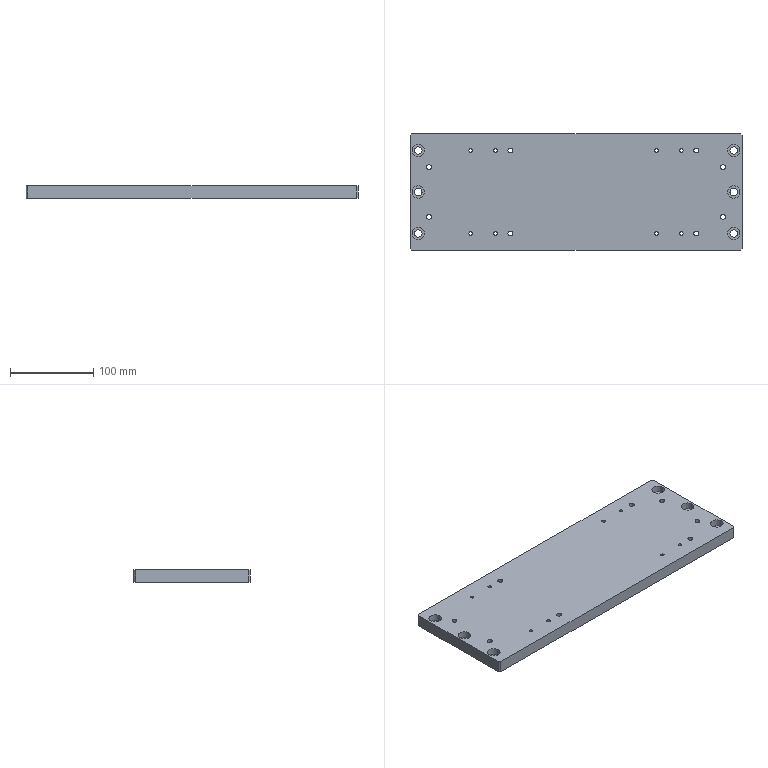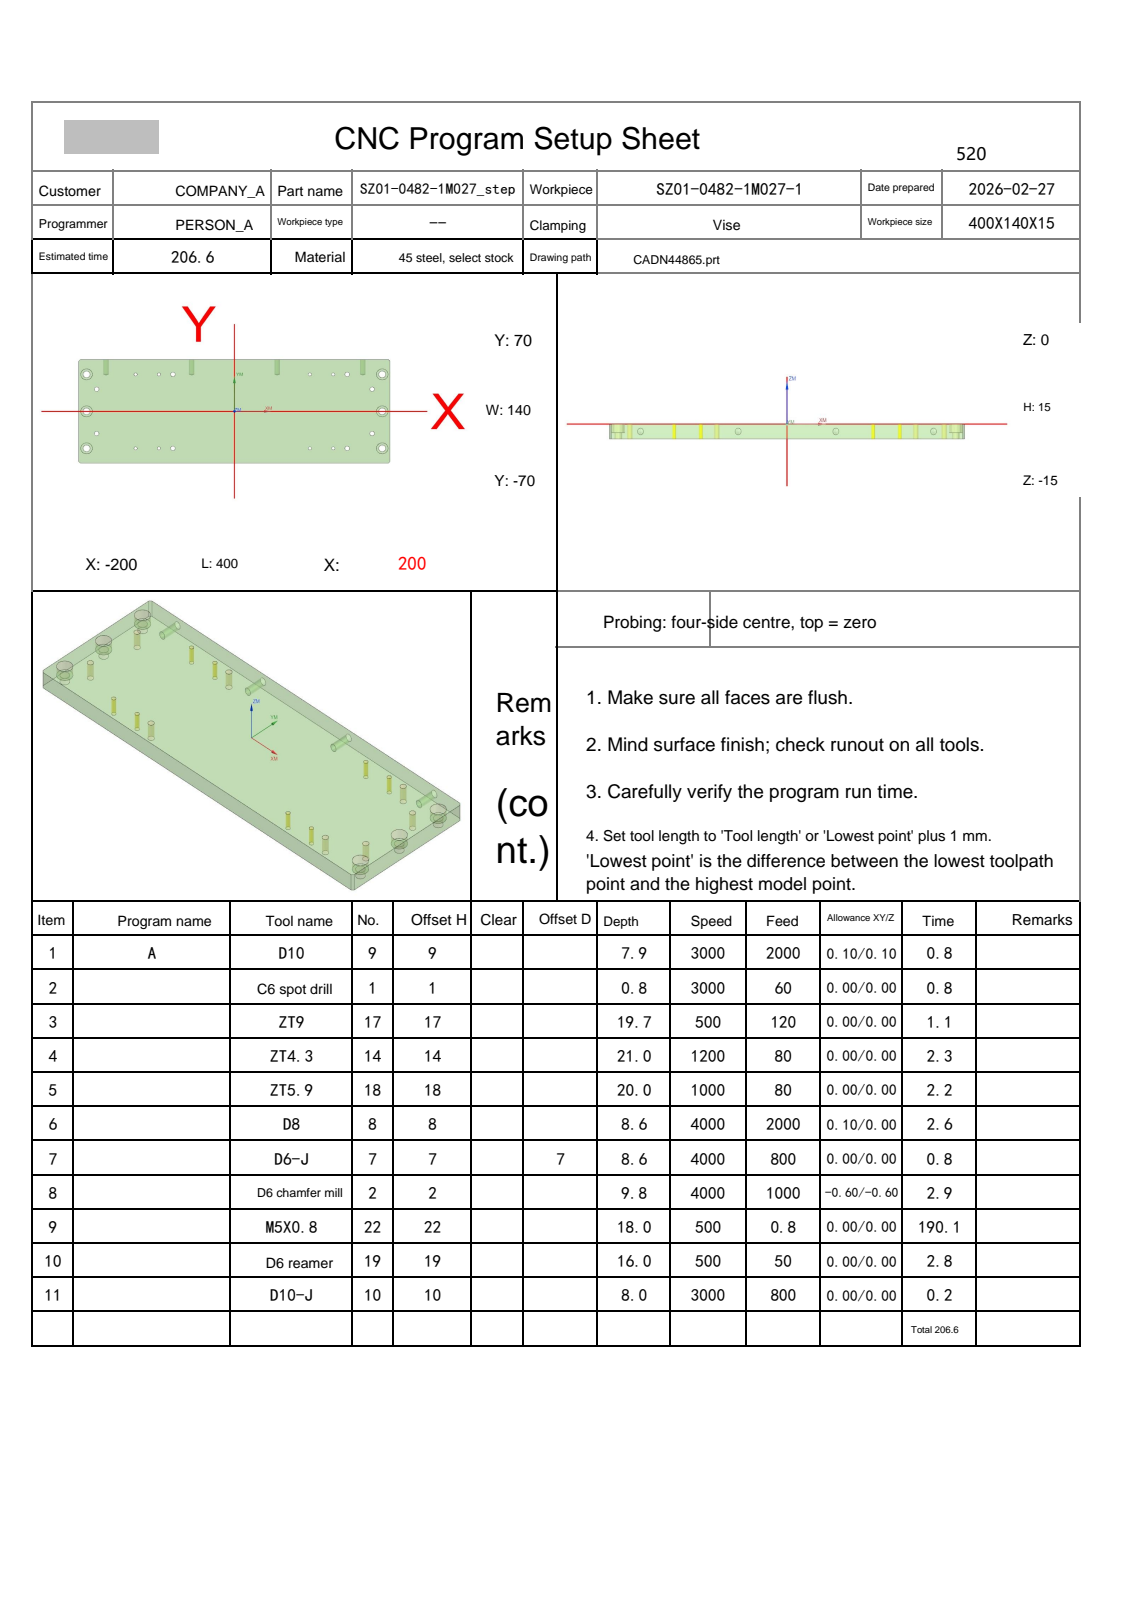NC program | NX | posted by the shop | part box 400 x 140 x 15 mm
Whole program:
%
O0001
(Machine time: 388.35 MIN)
(===Total Tool:11===)
(T9=D10     D=10.  R=0.   D-  H09 Z=-7.9  )
(T1=C6 spot drill   D=6.   R=0.   D-  H01 Z=-0.8  )
(T17=ZT9    D=9.   DR_a=118 D-  H17 Z=-19.7 )
(T14=ZT4.3  D=4.3  DR_a=118 D-  H14 Z=-21.  )
(T18=ZT5.9  D=5.9  DR_a=120 D-  H18 Z=-20.  )
(T8=D8      D=8.   R=0.   D-  H08 Z=-8.6  )
(T7=D6-J    D=6.   R=0.   D7  H07 Z=-8.6  )
(T2=D6 chamfer mill   D=6.   R=0.   D-  H02 Z=-9.8  )
(T22=M5X0.8 D=4.2  DR_a=180 D-  H22 Z=-18.  )
(T19=D6 reamer   D=6.   DR_a=180 D-  H19 Z=-16.  )
(T10=D10-J  D=10.  R=0.   D-  H10 Z=-8.   )
G80 G90 G17 G49 G40
G91 G28 Z0
M01
N1 T09 M06
(D10  D=10. R=0. H=09 ce=0.10 di=0.10)
G00 G90 G54 X195.242 Y79.97 M03 S3000
G43 H09 Z50.
M08
Z-.5
G01 X201.606 Y73.606 F2000.
X203.606 Y71.606
X209.97 Y65.242
G00 Z-1.
G01 X203.606 Y71.606
X201.606 Y73.606
X195.242 Y79.97
G00 Z-1.5
G01 X201.606 Y73.606
X203.606 Y71.606
X209.97 Y65.242
G00 Z-2.
G01 X203.606 Y71.606
X201.606 Y73.606
X195.242 Y79.97
G00 Z-2.5
G01 X201.606 Y73.606
X203.606 Y71.606
X209.97 Y65.242
G00 Z-3.
G01 X203.606 Y71.606
X201.606 Y73.606
X195.242 Y79.97
G00 Z-3.5
G01 X201.606 Y73.606
X203.606 Y71.606
X209.97 Y65.242
G00 Z-4.
G01 X203.606 Y71.606
X201.606 Y73.606
X195.242 Y79.97
G00 Z-4.5
G01 X201.606 Y73.606
X203.606 Y71.606
X209.97 Y65.242
G00 Z-5.
G01 X203.606 Y71.606
X201.606 Y73.606
X195.242 Y79.97
G00 Z-5.5
G01 X201.606 Y73.606
X203.606 Y71.606
X209.97 Y65.242
G00 Z-6.
G01 X203.606 Y71.606
X201.606 Y73.606
X195.242 Y79.97
G00 Z-6.5
G01 X201.606 Y73.606
X203.606 Y71.606
X209.97 Y65.242
G00 Z-7.
G01 X203.606 Y71.606
X201.606 Y73.606
X195.242 Y79.97
G00 Z-7.5
G01 X201.606 Y73.606
X203.606 Y71.606
X209.97 Y65.242
G00 Z-7.9
G01 X203.606 Y71.606
X201.606 Y73.606
X195.242 Y79.97
G00 Z50.
X209.97 Y-65.242
Z-.5
G01 X203.606 Y-71.606
X201.606 Y-73.606
X195.242 Y-79.97
G00 Z-1.
G01 X201.606 Y-73.606
X203.606 Y-71.606
X209.97 Y-65.242
G00 Z-1.5
G01 X203.606 Y-71.606
X201.606 Y-73.606
X195.242 Y-79.97
G00 Z-2.
G01 X201.606 Y-73.606
X203.606 Y-71.606
X209.97 Y-65.242
G00 Z-2.5
G01 X203.606 Y-71.606
X201.606 Y-73.606
X195.242 Y-79.97
G00 Z-3.
G01 X201.606 Y-73.606
X203.606 Y-71.606
X209.97 Y-65.242
G00 Z-3.5
G01 X203.606 Y-71.606
X201.606 Y-73.606
X195.242 Y-79.97
G00 Z-4.
G01 X201.606 Y-73.606
X203.606 Y-71.606
X209.97 Y-65.242
G00 Z-4.5
G01 X203.606 Y-71.606
X201.606 Y-73.606
X195.242 Y-79.97
G00 Z-5.
G01 X201.606 Y-73.606
X203.606 Y-71.606
X209.97 Y-65.242
G00 Z-5.5
G01 X203.606 Y-71.606
X201.606 Y-73.606
X195.242 Y-79.97
G00 Z-6.
G01 X201.606 Y-73.606
X203.606 Y-71.606
X209.97 Y-65.242
G00 Z-6.5
G01 X203.606 Y-71.606
X201.606 Y-73.606
X195.242 Y-79.97
G00 Z-7.
G01 X201.606 Y-73.606
X203.606 Y-71.606
X209.97 Y-65.242
G00 Z-7.5
G01 X203.606 Y-71.606
X201.606 Y-73.606
X195.242 Y-79.97
G00 Z-7.9
G01 X201.606 Y-73.606
X203.606 Y-71.606
X209.97 Y-65.242
G00 Z50.
X-195.242 Y-79.97
Z-.5
G01 X-201.606 Y-73.606
X-203.606 Y-71.606
X-209.97 Y-65.242
G00 Z-1.
G01 X-203.606 Y-71.606
X-201.606 Y-73.606
X-195.242 Y-79.97
G00 Z-1.5
G01 X-201.606 Y-73.606
X-203.606 Y-71.606
X-209.97 Y-65.242
G00 Z-2.
G01 X-203.606 Y-71.606
X-201.606 Y-73.606
X-195.242 Y-79.97
G00 Z-2.5
G01 X-201.606 Y-73.606
X-203.606 Y-71.606
X-209.97 Y-65.242
G00 Z-3.
G01 X-203.606 Y-71.606
X-201.606 Y-73.606
X-195.242 Y-79.97
G00 Z-3.5
G01 X-201.606 Y-73.606
X-203.606 Y-71.606
X-209.97 Y-65.242
G00 Z-4.
G01 X-203.606 Y-71.606
X-201.606 Y-73.606
X-195.242 Y-79.97
G00 Z-4.5
G01 X-201.606 Y-73.606
X-203.606 Y-71.606
X-209.97 Y-65.242
G00 Z-5.
G01 X-203.606 Y-71.606
X-201.606 Y-73.606
X-195.242 Y-79.97
G00 Z-5.5
G01 X-201.606 Y-73.606
X-203.606 Y-71.606
X-209.97 Y-65.242
G00 Z-6.
G01 X-203.606 Y-71.606
X-201.606 Y-73.606
X-195.242 Y-79.97
G00 Z-6.5
G01 X-201.606 Y-73.606
X-203.606 Y-71.606
X-209.97 Y-65.242
G00 Z-7.
G01 X-203.606 Y-71.606
X-201.606 Y-73.606
X-195.242 Y-79.97
G00 Z-7.5
G01 X-201.606 Y-73.606
X-203.606 Y-71.606
X-209.97 Y-65.242
G00 Z-7.9
G01 X-203.606 Y-71.606
X-201.606 Y-73.606
X-195.242 Y-79.97
G00 Z50.
X-209.97 Y65.242
Z-.5
G01 X-203.606 Y71.606
X-201.606 Y73.606
X-195.242 Y79.97
G00 Z-1.
G01 X-201.606 Y73.606
X-203.606 Y71.606
X-209.97 Y65.242
G00 Z-1.5
G01 X-203.606 Y71.606
X-201.606 Y73.606
X-195.242 Y79.97
G00 Z-2.
G01 X-201.606 Y73.606
X-203.606 Y71.606
X-209.97 Y65.242
G00 Z-2.5
G01 X-203.606 Y71.606
X-201.606 Y73.606
X-195.242 Y79.97
G00 Z-3.
G01 X-201.606 Y73.606
X-203.606 Y71.606
X-209.97 Y65.242
G00 Z-3.5
G01 X-203.606 Y71.606
X-201.606 Y73.606
X-195.242 Y79.97
G00 Z-4.
G01 X-201.606 Y73.606
X-203.606 Y71.606
X-209.97 Y65.242
G00 Z-4.5
G01 X-203.606 Y71.606
X-201.606 Y73.606
X-195.242 Y79.97
G00 Z-5.
G01 X-201.606 Y73.606
X-203.606 Y71.606
X-209.97 Y65.242
G00 Z-5.5
G01 X-203.606 Y71.606
X-201.606 Y73.606
X-195.242 Y79.97
G00 Z-6.
G01 X-201.606 Y73.606
X-203.606 Y71.606
X-209.97 Y65.242
G00 Z-6.5
G01 X-203.606 Y71.606
X-201.606 Y73.606
X-195.242 Y79.97
G00 Z-7.
G01 X-201.606 Y73.606
X-203.606 Y71.606
X-209.97 Y65.242
G00 Z-7.5
G01 X-203.606 Y71.606
X-201.606 Y73.606
X-195.242 Y79.97
G00 Z-7.9
G01 X-201.606 Y73.606
X-203.606 Y71.606
X-209.97 Y65.242
G00 Z50.
G91 G28 Z0.0
M05
M09
G91 G28 Z0.0
M01
N2 T01 M06
(C6 spot drill  D=6. R=0. H=01 ce=0.00 di=0.10)
G00 G90 G54 X97. Y50. M03 S3000
G43 H01 Z50.
M08
G98 G81 X97. Y50. Z-.8 R1. F60.
X127.
X145.
X190.
X177. Y30.
X190. Y0.0
X177. Y-30.
X190. Y-50.
X145.
X127.
X97.
X-79.
X-97.
X-127.
X-190.
X-177. Y-30.
X-190. Y0.0
X-177. Y30.
X-190. Y50.
X-127.
X-97.
X-79.
G80
G00 Z50.
G91 G28 Z0.0
M05
M09
G91 G28 Z0.0
M01
N3 T17 M06
(ZT9 D=9. DR_a=118 H=17)
G00 G90 G54 X-190. Y-50. M03 S500
G43 H17 Z50.
M08
G98 G83 X-190. Y-50. Z-19.704 R1. F120. Q2.
Y0.0
Y50.
X190.
Y0.0
Y-50.
G80
G00 Z50.
G91 G28 Z0.0
M05
M09
G91 G28 Z0.0
M01
N4 T14 M06
(ZT4.3 D=4.3 DR_a=118 H=14)
G00 G90 G54 X97. Y-50. M03 S1200
G43 H14 Z50.
M08
G98 G83 X97. Y-50. Z-21. R1. F80. Q1.5
X127.
Y50.
X97.
X-97.
X-127.
Y-50.
X-97.
G80
G00 Z50.
G91 G28 Z0.0
M05
M09
G91 G28 Z0.0
M01
N5 T18 M06
(ZT5.9 D=5.9 DR_a=120 H=18)
G00 G90 G54 X145. Y-50. M03 S1000
G43 H18 Z50.
M08
G98 G83 X145. Y-50. Z-20. R1. F80. Q1.
X177. Y-30.
Y30.
X145. Y50.
X-79.
Y-50.
X-177. Y-30.
Y30.
G80
G00 Z50.
G91 G28 Z0.0
M05
M09
G91 G28 Z0.0
M01
N6 T08 M06
(D8  D=8. R=0. H=08 ce=0.10 di=0.00)
G00 G90 G54 X190. Y0.0 M03 S4000
G43 H08 Z50.
M08
Z.5
G03 X191.7 Y-1.7 I1.7 J0.0 F2000.
X193.4 Y0.0 I0.0 J1.7
X193.4 Y0.0 Z.25 I-3.4 J0.0
X193.4 Y0.0 Z0.0 I-3.4 J0.0
X193.4 Y0.0 Z-.25 I-3.4 J0.0
X193.4 Y0.0 Z-.5 I-3.4 J0.0
X193.4 Y0.0 Z-.75 I-3.4 J0.0
X193.4 Y0.0 Z-1. I-3.4 J0.0
X193.4 Y0.0 Z-1.25 I-3.4 J0.0
X193.4 Y0.0 Z-1.5 I-3.4 J0.0
X193.4 Y0.0 Z-1.75 I-3.4 J0.0
X193.4 Y0.0 Z-2. I-3.4 J0.0
X193.4 Y0.0 Z-2.25 I-3.4 J0.0
X193.4 Y0.0 Z-2.5 I-3.4 J0.0
X193.4 Y0.0 Z-2.75 I-3.4 J0.0
X193.4 Y0.0 Z-3. I-3.4 J0.0
X193.4 Y0.0 Z-3.25 I-3.4 J0.0
X193.4 Y0.0 Z-3.5 I-3.4 J0.0
X193.4 Y0.0 Z-3.75 I-3.4 J0.0
X193.4 Y0.0 Z-4. I-3.4 J0.0
X193.4 Y0.0 Z-4.25 I-3.4 J0.0
X193.4 Y0.0 Z-4.5 I-3.4 J0.0
X193.4 Y0.0 Z-4.75 I-3.4 J0.0
X193.4 Y0.0 Z-5. I-3.4 J0.0
X193.4 Y0.0 Z-5.25 I-3.4 J0.0
X193.4 Y0.0 Z-5.5 I-3.4 J0.0
X193.4 Y0.0 Z-5.75 I-3.4 J0.0
X193.4 Y0.0 Z-6. I-3.4 J0.0
X193.4 Y0.0 Z-6.25 I-3.4 J0.0
X193.4 Y0.0 Z-6.5 I-3.4 J0.0
X193.4 Y0.0 Z-6.75 I-3.4 J0.0
X193.4 Y0.0 Z-7. I-3.4 J0.0
X193.4 Y0.0 Z-7.25 I-3.4 J0.0
X193.4 Y0.0 Z-7.5 I-3.4 J0.0
X193.4 Y0.0 Z-7.75 I-3.4 J0.0
X193.4 Y0.0 Z-8. I-3.4 J0.0
X193.4 Y0.0 Z-8.25 I-3.4 J0.0
X193.4 Y0.0 Z-8.5 I-3.4 J0.0
X187.249 Y1.998 Z-8.6 I-3.4 J0.0
X186.6 Y0.0 I2.751 J-1.998
X190. Y-3.4 I3.4 J0.0
X193.4 Y0.0 I0.0 J3.4
X190. Y3.4 I-3.4 J0.0
X187.249 Y1.998 I0.0 J-3.4
X186.925 Y.999 I1.375 J-.999
X188.625 Y-.701 I1.7 J0.0
X190. Y0.0 I0.0 J1.7
G00 Z50.
Y-50.
Z.5
G03 X191.7 Y-51.7 I1.7 J0.0
X193.4 Y-50. I0.0 J1.7
X193.4 Y-50. Z.25 I-3.4 J0.0
X193.4 Y-50. Z0.0 I-3.4 J0.0
X193.4 Y-50. Z-.25 I-3.4 J0.0
X193.4 Y-50. Z-.5 I-3.4 J0.0
X193.4 Y-50. Z-.75 I-3.4 J0.0
X193.4 Y-50. Z-1. I-3.4 J0.0
X193.4 Y-50. Z-1.25 I-3.4 J0.0
X193.4 Y-50. Z-1.5 I-3.4 J0.0
X193.4 Y-50. Z-1.75 I-3.4 J0.0
X193.4 Y-50. Z-2. I-3.4 J0.0
X193.4 Y-50. Z-2.25 I-3.4 J0.0
X193.4 Y-50. Z-2.5 I-3.4 J0.0
X193.4 Y-50. Z-2.75 I-3.4 J0.0
X193.4 Y-50. Z-3. I-3.4 J0.0
X193.4 Y-50. Z-3.25 I-3.4 J0.0
X193.4 Y-50. Z-3.5 I-3.4 J0.0
X193.4 Y-50. Z-3.75 I-3.4 J0.0
X193.4 Y-50. Z-4. I-3.4 J0.0
X193.4 Y-50. Z-4.25 I-3.4 J0.0
X193.4 Y-50. Z-4.5 I-3.4 J0.0
X193.4 Y-50. Z-4.75 I-3.4 J0.0
X193.4 Y-50. Z-5. I-3.4 J0.0
X193.4 Y-50. Z-5.25 I-3.4 J0.0
X193.4 Y-50. Z-5.5 I-3.4 J0.0
X193.4 Y-50. Z-5.75 I-3.4 J0.0
X193.4 Y-50. Z-6. I-3.4 J0.0
X193.4 Y-50. Z-6.25 I-3.4 J0.0
X193.4 Y-50. Z-6.5 I-3.4 J0.0
X193.4 Y-50. Z-6.75 I-3.4 J0.0
X193.4 Y-50. Z-7. I-3.4 J0.0
X193.4 Y-50. Z-7.25 I-3.4 J0.0
X193.4 Y-50. Z-7.5 I-3.4 J0.0
X193.4 Y-50. Z-7.75 I-3.4 J0.0
X193.4 Y-50. Z-8. I-3.4 J0.0
X193.4 Y-50. Z-8.25 I-3.4 J0.0
X193.4 Y-50. Z-8.5 I-3.4 J0.0
X187.249 Y-48.002 Z-8.6 I-3.4 J0.0
X186.6 Y-50. I2.751 J-1.998
X190. Y-53.4 I3.4 J0.0
X193.4 Y-50. I0.0 J3.4
X190. Y-46.6 I-3.4 J0.0
X187.249 Y-48.002 I0.0 J-3.4
X186.925 Y-49.001 I1.375 J-.999
X188.625 Y-50.701 I1.7 J0.0
X190. Y-50. I0.0 J1.7
G00 Z50.
Y50.
Z.5
G03 X191.7 Y48.3 I1.7 J0.0
X193.4 Y50. I0.0 J1.7
X193.4 Y50. Z.25 I-3.4 J0.0
X193.4 Y50. Z0.0 I-3.4 J0.0
X193.4 Y50. Z-.25 I-3.4 J0.0
X193.4 Y50. Z-.5 I-3.4 J0.0
X193.4 Y50. Z-.75 I-3.4 J0.0
X193.4 Y50. Z-1. I-3.4 J0.0
X193.4 Y50. Z-1.25 I-3.4 J0.0
X193.4 Y50. Z-1.5 I-3.4 J0.0
X193.4 Y50. Z-1.75 I-3.4 J0.0
X193.4 Y50. Z-2. I-3.4 J0.0
X193.4 Y50. Z-2.25 I-3.4 J0.0
X193.4 Y50. Z-2.5 I-3.4 J0.0
X193.4 Y50. Z-2.75 I-3.4 J0.0
X193.4 Y50. Z-3. I-3.4 J0.0
X193.4 Y50. Z-3.25 I-3.4 J0.0
X193.4 Y50. Z-3.5 I-3.4 J0.0
X193.4 Y50. Z-3.75 I-3.4 J0.0
X193.4 Y50. Z-4. I-3.4 J0.0
X193.4 Y50. Z-4.25 I-3.4 J0.0
X193.4 Y50. Z-4.5 I-3.4 J0.0
X193.4 Y50. Z-4.75 I-3.4 J0.0
X193.4 Y50. Z-5. I-3.4 J0.0
X193.4 Y50. Z-5.25 I-3.4 J0.0
X193.4 Y50. Z-5.5 I-3.4 J0.0
X193.4 Y50. Z-5.75 I-3.4 J0.0
X193.4 Y50. Z-6. I-3.4 J0.0
X193.4 Y50. Z-6.25 I-3.4 J0.0
X193.4 Y50. Z-6.5 I-3.4 J0.0
X193.4 Y50. Z-6.75 I-3.4 J0.0
X193.4 Y50. Z-7. I-3.4 J0.0
X193.4 Y50. Z-7.25 I-3.4 J0.0
X193.4 Y50. Z-7.5 I-3.4 J0.0
X193.4 Y50. Z-7.75 I-3.4 J0.0
X193.4 Y50. Z-8. I-3.4 J0.0
X193.4 Y50. Z-8.25 I-3.4 J0.0
X193.4 Y50. Z-8.5 I-3.4 J0.0
X187.249 Y51.998 Z-8.6 I-3.4 J0.0
X186.6 Y50. I2.751 J-1.998
X190. Y46.6 I3.4 J0.0
X193.4 Y50. I0.0 J3.4
X190. Y53.4 I-3.4 J0.0
X187.249 Y51.998 I0.0 J-3.4
X186.925 Y50.999 I1.375 J-.999
X188.625 Y49.299 I1.7 J0.0
X190. Y50. I0.0 J1.7
G00 Z50.
X-190.
Z.5
G03 X-188.3 Y48.3 I1.7 J0.0
X-186.6 Y50. I0.0 J1.7
X-186.6 Y50. Z.25 I-3.4 J0.0
X-186.6 Y50. Z0.0 I-3.4 J0.0
X-186.6 Y50. Z-.25 I-3.4 J0.0
X-186.6 Y50. Z-.5 I-3.4 J0.0
X-186.6 Y50. Z-.75 I-3.4 J0.0
X-186.6 Y50. Z-1. I-3.4 J0.0
X-186.6 Y50. Z-1.25 I-3.4 J0.0
X-186.6 Y50. Z-1.5 I-3.4 J0.0
X-186.6 Y50. Z-1.75 I-3.4 J0.0
X-186.6 Y50. Z-2. I-3.4 J0.0
X-186.6 Y50. Z-2.25 I-3.4 J0.0
X-186.6 Y50. Z-2.5 I-3.4 J0.0
X-186.6 Y50. Z-2.75 I-3.4 J0.0
X-186.6 Y50. Z-3. I-3.4 J0.0
X-186.6 Y50. Z-3.25 I-3.4 J0.0
X-186.6 Y50. Z-3.5 I-3.4 J0.0
X-186.6 Y50. Z-3.75 I-3.4 J0.0
X-186.6 Y50. Z-4. I-3.4 J0.0
X-186.6 Y50. Z-4.25 I-3.4 J0.0
X-186.6 Y50. Z-4.5 I-3.4 J0.0
X-186.6 Y50. Z-4.75 I-3.4 J0.0
X-186.6 Y50. Z-5. I-3.4 J0.0
X-186.6 Y50. Z-5.25 I-3.4 J0.0
X-186.6 Y50. Z-5.5 I-3.4 J0.0
X-186.6 Y50. Z-5.75 I-3.4 J0.0
X-186.6 Y50. Z-6. I-3.4 J0.0
X-186.6 Y50. Z-6.25 I-3.4 J0.0
X-186.6 Y50. Z-6.5 I-3.4 J0.0
X-186.6 Y50. Z-6.75 I-3.4 J0.0
X-186.6 Y50. Z-7. I-3.4 J0.0
X-186.6 Y50. Z-7.25 I-3.4 J0.0
X-186.6 Y50. Z-7.5 I-3.4 J0.0
X-186.6 Y50. Z-7.75 I-3.4 J0.0
X-186.6 Y50. Z-8. I-3.4 J0.0
X-186.6 Y50. Z-8.25 I-3.4 J0.0
X-186.6 Y50. Z-8.5 I-3.4 J0.0
X-192.751 Y51.998 Z-8.6 I-3.4 J0.0
X-193.4 Y50. I2.751 J-1.998
X-190. Y46.6 I3.4 J0.0
X-186.6 Y50. I0.0 J3.4
X-190. Y53.4 I-3.4 J0.0
X-192.751 Y51.998 I0.0 J-3.4
X-193.075 Y50.999 I1.375 J-.999
X-191.375 Y49.299 I1.7 J0.0
X-190. Y50. I0.0 J1.7
G00 Z50.
Y0.0
Z.5
G03 X-188.3 Y-1.7 I1.7 J0.0
X-186.6 Y0.0 I0.0 J1.7
X-186.6 Y0.0 Z.25 I-3.4 J0.0
X-186.6 Y0.0 Z0.0 I-3.4 J0.0
X-186.6 Y0.0 Z-.25 I-3.4 J0.0
X-186.6 Y0.0 Z-.5 I-3.4 J0.0
X-186.6 Y0.0 Z-.75 I-3.4 J0.0
X-186.6 Y0.0 Z-1. I-3.4 J0.0
X-186.6 Y0.0 Z-1.25 I-3.4 J0.0
X-186.6 Y0.0 Z-1.5 I-3.4 J0.0
X-186.6 Y0.0 Z-1.75 I-3.4 J0.0
X-186.6 Y0.0 Z-2. I-3.4 J0.0
X-186.6 Y0.0 Z-2.25 I-3.4 J0.0
X-186.6 Y0.0 Z-2.5 I-3.4 J0.0
X-186.6 Y0.0 Z-2.75 I-3.4 J0.0
X-186.6 Y0.0 Z-3. I-3.4 J0.0
X-186.6 Y0.0 Z-3.25 I-3.4 J0.0
X-186.6 Y0.0 Z-3.5 I-3.4 J0.0
X-186.6 Y0.0 Z-3.75 I-3.4 J0.0
X-186.6 Y0.0 Z-4. I-3.4 J0.0
X-186.6 Y0.0 Z-4.25 I-3.4 J0.0
X-186.6 Y0.0 Z-4.5 I-3.4 J0.0
X-186.6 Y0.0 Z-4.75 I-3.4 J0.0
X-186.6 Y0.0 Z-5. I-3.4 J0.0
X-186.6 Y0.0 Z-5.25 I-3.4 J0.0
X-186.6 Y0.0 Z-5.5 I-3.4 J0.0
X-186.6 Y0.0 Z-5.75 I-3.4 J0.0
X-186.6 Y0.0 Z-6. I-3.4 J0.0
X-186.6 Y0.0 Z-6.25 I-3.4 J0.0
X-186.6 Y0.0 Z-6.5 I-3.4 J0.0
X-186.6 Y0.0 Z-6.75 I-3.4 J0.0
X-186.6 Y0.0 Z-7. I-3.4 J0.0
X-186.6 Y0.0 Z-7.25 I-3.4 J0.0
X-186.6 Y0.0 Z-7.5 I-3.4 J0.0
X-186.6 Y0.0 Z-7.75 I-3.4 J0.0
X-186.6 Y0.0 Z-8. I-3.4 J0.0
X-186.6 Y0.0 Z-8.25 I-3.4 J0.0
X-186.6 Y0.0 Z-8.5 I-3.4 J0.0
X-192.751 Y1.998 Z-8.6 I-3.4 J0.0
X-193.4 Y0.0 I2.751 J-1.998
X-190. Y-3.4 I3.4 J0.0
X-186.6 Y0.0 I0.0 J3.4
X-190. Y3.4 I-3.4 J0.0
X-192.751 Y1.998 I0.0 J-3.4
X-193.075 Y.999 I1.375 J-.999
X-191.375 Y-.701 I1.7 J0.0
X-190. Y0.0 I0.0 J1.7
G00 Z50.
Y-50.
Z.5
G03 X-188.3 Y-51.7 I1.7 J0.0
X-186.6 Y-50. I0.0 J1.7
X-186.6 Y-50. Z.25 I-3.4 J0.0
X-186.6 Y-50. Z0.0 I-3.4 J0.0
X-186.6 Y-50. Z-.25 I-3.4 J0.0
X-186.6 Y-50. Z-.5 I-3.4 J0.0
X-186.6 Y-50. Z-.75 I-3.4 J0.0
X-186.6 Y-50. Z-1. I-3.4 J0.0
X-186.6 Y-50. Z-1.25 I-3.4 J0.0
X-186.6 Y-50. Z-1.5 I-3.4 J0.0
X-186.6 Y-50. Z-1.75 I-3.4 J0.0
X-186.6 Y-50. Z-2. I-3.4 J0.0
X-186.6 Y-50. Z-2.25 I-3.4 J0.0
X-186.6 Y-50. Z-2.5 I-3.4 J0.0
X-186.6 Y-50. Z-2.75 I-3.4 J0.0
X-186.6 Y-50. Z-3. I-3.4 J0.0
X-186.6 Y-50. Z-3.25 I-3.4 J0.0
X-186.6 Y-50. Z-3.5 I-3.4 J0.0
X-186.6 Y-50. Z-3.75 I-3.4 J0.0
X-186.6 Y-50. Z-4. I-3.4 J0.0
X-186.6 Y-50. Z-4.25 I-3.4 J0.0
X-186.6 Y-50. Z-4.5 I-3.4 J0.0
X-186.6 Y-50. Z-4.75 I-3.4 J0.0
X-186.6 Y-50. Z-5. I-3.4 J0.0
X-186.6 Y-50. Z-5.25 I-3.4 J0.0
X-186.6 Y-50. Z-5.5 I-3.4 J0.0
X-186.6 Y-50. Z-5.75 I-3.4 J0.0
X-186.6 Y-50. Z-6. I-3.4 J0.0
X-186.6 Y-50. Z-6.25 I-3.4 J0.0
X-186.6 Y-50. Z-6.5 I-3.4 J0.0
X-186.6 Y-50. Z-6.75 I-3.4 J0.0
X-186.6 Y-50. Z-7. I-3.4 J0.0
X-186.6 Y-50. Z-7.25 I-3.4 J0.0
X-186.6 Y-50. Z-7.5 I-3.4 J0.0
X-186.6 Y-50. Z-7.75 I-3.4 J0.0
X-186.6 Y-50. Z-8. I-3.4 J0.0
X-186.6 Y-50. Z-8.25 I-3.4 J0.0
X-186.6 Y-50. Z-8.5 I-3.4 J0.0
X-192.751 Y-48.002 Z-8.6 I-3.4 J0.0
X-193.4 Y-50. I2.751 J-1.998
X-190. Y-53.4 I3.4 J0.0
X-186.6 Y-50. I0.0 J3.4
X-190. Y-46.6 I-3.4 J0.0
X-192.751 Y-48.002 I0.0 J-3.4
X-193.075 Y-49.001 I1.375 J-.999
X-191.375 Y-50.701 I1.7 J0.0
X-190. Y-50. I0.0 J1.7
G00 Z50.
G91 G28 Z0.0
M05
M09
G91 G28 Z0.0
M01
N7 T07 M06
(D6-J  D=6. R=0. H=07 ce=0.00 di=0.00)
G00 G90 G54 X190. Y0.0 M03 S4000
G43 H07 Z50.
M08
Z.5
G41 D07
G01 X190.794 Y-1.153 F800.
G03 X192.468 Y-2.032 I1.674 J1.153
X194.5 Y0.0 I0.0 J2.032
X194.5 Y0.0 Z-4.5 I-4.5 J0.0
X191.916 Y-4.072 Z-8.6 I-4.5 J0.0
X194.5 Y0.0 I-1.916 J4.072
X190. Y4.5 I-4.5 J0.0
X185.5 Y0.0 I0.0 J-4.5
X190. Y-4.5 I4.5 J0.0
X191.916 Y-4.072 I0.0 J4.5
X193.083 Y-2.233 I-.865 J1.839
X191.381 Y-.228 I-2.032 J0.0
G01 G40 X190. Y0.0
G00 Z50.
Y-50.
Z.5
G41 D07
G01 X190.794 Y-51.153
G03 X192.468 Y-52.032 I1.674 J1.153
X194.5 Y-50. I0.0 J2.032
X194.5 Y-50. Z-4.5 I-4.5 J0.0
X191.916 Y-54.072 Z-8.6 I-4.5 J0.0
X194.5 Y-50. I-1.916 J4.072
X190. Y-45.5 I-4.5 J0.0
X185.5 Y-50. I0.0 J-4.5
X190. Y-54.5 I4.5 J0.0
X191.916 Y-54.072 I0.0 J4.5
X193.083 Y-52.233 I-.865 J1.839
X191.381 Y-50.228 I-2.032 J0.0
G01 G40 X190. Y-50.
G00 Z50.
Y50.
Z.5
G41 D07
G01 X190.794 Y48.847
G03 X192.468 Y47.968 I1.674 J1.153
X194.5 Y50. I0.0 J2.032
X194.5 Y50. Z-4.5 I-4.5 J0.0
X191.916 Y45.928 Z-8.6 I-4.5 J0.0
X194.5 Y50. I-1.916 J4.072
X190. Y54.5 I-4.5 J0.0
X185.5 Y50. I0.0 J-4.5
X190. Y45.5 I4.5 J0.0
X191.916 Y45.928 I0.0 J4.5
X193.083 Y47.767 I-.865 J1.839
X191.381 Y49.772 I-2.032 J0.0
G01 G40 X190. Y50.
G00 Z50.
X-190.
Z.5
G41 D07
G01 X-189.206 Y48.847
G03 X-187.532 Y47.968 I1.674 J1.153
X-185.5 Y50. I0.0 J2.032
X-185.5 Y50. Z-4.5 I-4.5 J0.0
X-188.084 Y45.928 Z-8.6 I-4.5 J0.0
X-185.5 Y50. I-1.916 J4.072
X-190. Y54.5 I-4.5 J0.0
X-194.5 Y50. I0.0 J-4.5
X-190. Y45.5 I4.5 J0.0
X-188.084 Y45.928 I0.0 J4.5
X-186.917 Y47.767 I-.865 J1.839
X-188.619 Y49.772 I-2.032 J0.0
G01 G40 X-190. Y50.
G00 Z50.
Y0.0
Z.5
G41 D07
G01 X-189.206 Y-1.153
G03 X-187.532 Y-2.032 I1.674 J1.153
X-185.5 Y0.0 I0.0 J2.032
X-185.5 Y0.0 Z-4.5 I-4.5 J0.0
X-188.084 Y-4.072 Z-8.6 I-4.5 J0.0
X-185.5 Y0.0 I-1.916 J4.072
X-190. Y4.5 I-4.5 J0.0
X-194.5 Y0.0 I0.0 J-4.5
X-190. Y-4.5 I4.5 J0.0
X-188.084 Y-4.072 I0.0 J4.5
X-186.917 Y-2.233 I-.865 J1.839
X-188.619 Y-.228 I-2.032 J0.0
G01 G40 X-190. Y0.0
G00 Z50.
Y-50.
Z.5
G41 D07
G01 X-189.206 Y-51.153
G03 X-187.532 Y-52.032 I1.674 J1.153
X-185.5 Y-50. I0.0 J2.032
X-185.5 Y-50. Z-4.5 I-4.5 J0.0
X-188.084 Y-54.072 Z-8.6 I-4.5 J0.0
X-185.5 Y-50. I-1.916 J4.072
X-190. Y-45.5 I-4.5 J0.0
X-194.5 Y-50. I0.0 J-4.5
X-190. Y-54.5 I4.5 J0.0
X-188.084 Y-54.072 I0.0 J4.5
X-186.917 Y-52.233 I-.865 J1.839
X-188.619 Y-50.228 I-2.032 J0.0
G01 G40 X-190. Y-50.
G00 Z50.
G91 G28 Z0.0
M05
M09
G91 G28 Z0.0
M01
N8 T02 M06
(D6 chamfer mill  D=6. R=0. H=02 ce=-0.60 di=0.00)
G00 G90 G54 X-97.093 Y-49.306 M03 S4000
G43 H02 Z50.
M08
Z-.5
G01 Z-1. F200.
X-97.2 Y-48.5
G03 X-98.7 Y-50. I0.0 J-1.5
X-97. Y-51.7 I1.7 J0.0
X-95.3 Y-50. I0.0 J1.7
X-97. Y-48.3 I-1.7 J0.0
X-98.7 Y-50. I0.0 J-1.7
X-97.2 Y-51.5 I1.5 J0.0
G01 X-97.093 Y-50.694
Z-.5
G00 Z50.
X-127.093 Y-49.306
Z-.5
G01 Z-1.
X-127.2 Y-48.5
G03 X-128.7 Y-50. I0.0 J-1.5
X-127. Y-51.7 I1.7 J0.0
X-125.3 Y-50. I0.0 J1.7
X-127. Y-48.3 I-1.7 J0.0
X-128.7 Y-50. I0.0 J-1.7
X-127.2 Y-51.5 I1.5 J0.0
G01 X-127.093 Y-50.694
Z-.5
G00 Z50.
Y50.694
Z-.5
G01 Z-1.
X-127.2 Y51.5
G03 X-128.7 Y50. I0.0 J-1.5
X-127. Y48.3 I1.7 J0.0
X-125.3 Y50. I0.0 J1.7
X-127. Y51.7 I-1.7 J0.0
X-128.7 Y50. I0.0 J-1.7
X-127.2 Y48.5 I1.5 J0.0
G01 X-127.093 Y49.306
Z-.5
G00 Z50.
X-97.093 Y50.694
Z-.5
G01 Z-1.
X-97.2 Y51.5
G03 X-98.7 Y50. I0.0 J-1.5
X-97. Y48.3 I1.7 J0.0
X-95.3 Y50. I0.0 J1.7
X-97. Y51.7 I-1.7 J0.0
X-98.7 Y50. I0.0 J-1.7
X-97.2 Y48.5 I1.5 J0.0
G01 X-97.093 Y49.306
Z-.5
G00 Z50.
X96.907 Y50.694
Z-.5
G01 Z-1.
X96.8 Y51.5
G03 X95.3 Y50. I0.0 J-1.5
X97. Y48.3 I1.7 J0.0
X98.7 Y50. I0.0 J1.7
X97. Y51.7 I-1.7 J0.0
X95.3 Y50. I0.0 J-1.7
X96.8 Y48.5 I1.5 J0.0
G01 X96.907 Y49.306
Z-.5
G00 Z50.
X126.907 Y50.694
Z-.5
G01 Z-1.
X126.8 Y51.5
G03 X125.3 Y50. I0.0 J-1.5
X127. Y48.3 I1.7 J0.0
X128.7 Y50. I0.0 J1.7
X127. Y51.7 I-1.7 J0.0
X125.3 Y50. I0.0 J-1.7
X126.8 Y48.5 I1.5 J0.0
G01 X126.907 Y49.306
Z-.5
G00 Z50.
Y-49.306
Z-.5
G01 Z-1.
X126.8 Y-48.5
G03 X125.3 Y-50. I0.0 J-1.5
X127. Y-51.7 I1.7 J0.0
X128.7 Y-50. I0.0 J1.7
X127. Y-48.3 I-1.7 J0.0
X125.3 Y-50. I0.0 J-1.7
X126.8 Y-51.5 I1.5 J0.0
G01 X126.907 Y-50.694
Z-.5
G00 Z50.
X96.907 Y-49.306
Z-.5
G01 Z-1.
X96.8 Y-48.5
G03 X95.3 Y-50. I0.0 J-1.5
X97. Y-51.7 I1.7 J0.0
X98.7 Y-50. I0.0 J1.7
X97. Y-48.3 I-1.7 J0.0
X95.3 Y-50. I0.0 J-1.7
X96.8 Y-51.5 I1.5 J0.0
G01 X96.907 Y-50.694
Z-.5
G00 Z50.
G00 G90 X-.386 Y71.227 M03 S3500
Z50.
Z.172
G01 Z-1.2 F1000.
G03 X-.1 Y71.027 I1.286 J1.532
G01 X-.054 Y70.997
X0.0 Y71.
X198.
X198.259 Y70.966
X198.5 Y70.866
X198.707 Y70.707
X200.707 Y68.707
X200.866 Y68.5
X200.966 Y68.259
X201. Y68.
Y-68.
X200.966 Y-68.259
X200.866 Y-68.5
X200.707 Y-68.707
X198.707 Y-70.707
X198.5 Y-70.866
X198.259 Y-70.966
X198. Y-71.
X-198.
X-198.259 Y-70.966
X-198.5 Y-70.866
X-198.707 Y-70.707
X-200.707 Y-68.707
X-200.866 Y-68.5
X-200.966 Y-68.259
X-201. Y-68.
Y68.
X-200.966 Y68.259
X-200.866 Y68.5
X-200.707 Y68.707
X-198.707 Y70.707
X-198.5 Y70.866
X-198.259 Y70.966
X-198. Y71.
X0.0
X.054 Y70.997
X.1 Y71.027
G03 X.386 Y71.227 I-1. J1.732
G01 Z.172
G00 Z10.
X-196.294 Y-49.603
Z.21
G01 Z-1.2
G03 X-196.478 Y-49.899 I1.597 J-1.204
G01 X-196.506 Y-49.946
X-196.5 Y-50.
G03 X-190. Y-56.5 I6.5 J0.0
X-183.5 Y-50. I0.0 J6.5
X-190. Y-43.5 I-6.5 J0.0
X-196.5 Y-50. I0.0 J-6.5
G01 X-196.506 Y-50.054
X-196.478 Y-50.101
G03 X-196.294 Y-50.397 I1.782 J.908
G01 Z.21
G00 Z10.
X-178.808 Y-29.596
Z.257
G01 Z-1.2
G03 X-178.982 Y-29.898 I1.638 J-1.147
G01 X-179.008 Y-29.946
X-179. Y-30.
G03 X-177. Y-32. I2. J0.0
X-175. Y-30. I0.0 J2.
X-177. Y-28. I-2. J0.0
X-178.97 Y-29.653 I0.0 J-2.
G01 X-179. Y-30.
X-179.008 Y-30.054
X-178.982 Y-30.102
G03 X-178.808 Y-30.404 I1.813 J.845
G01 Z.257
G00 Z10.
X-196.294 Y.397
Z.21
G01 Z-1.2
G03 X-196.478 Y.101 I1.597 J-1.204
G01 X-196.506 Y.054
X-196.5 Y0.0
G03 X-190. Y-6.5 I6.5 J0.0
X-183.5 Y0.0 I0.0 J6.5
X-190. Y6.5 I-6.5 J0.0
X-196.5 Y0.0 I0.0 J-6.5
G01 X-196.506 Y-.054
X-196.478 Y-.101
G03 X-196.294 Y-.397 I1.782 J.908
G01 Z.21
G00 Z10.
X-178.808 Y30.404
Z.257
G01 Z-1.2
G03 X-178.982 Y30.102 I1.638 J-1.147
G01 X-179.008 Y30.054
X-179. Y30.
G03 X-177. Y28. I2. J0.0
X-175. Y30. I0.0 J2.
X-177. Y32. I-2. J0.0
X-178.97 Y30.347 I0.0 J-2.
G01 X-179. Y30.
X-179.008 Y29.946
X-178.982 Y29.898
G03 X-178.808 Y29.596 I1.813 J.845
G01 Z.257
G00 Z10.
X-196.294 Y50.397
Z.21
G01 Z-1.2
G03 X-196.478 Y50.101 I1.597 J-1.204
G01 X-196.506 Y50.054
X-196.5 Y50.
G03 X-190. Y43.5 I6.5 J0.0
X-183.5 Y50. I0.0 J6.5
X-190. Y56.5 I-6.5 J0.0
X-196.5 Y50. I0.0 J-6.5
G01 X-196.506 Y49.946
X-196.478 Y49.899
G03 X-196.294 Y49.603 I1.782 J.908
G01 Z.21
G00 Z10.
X-127.926 Y50.412
Z.32
G01 Z-1.2
G03 X-128.086 Y50.103 I1.687 J-1.075
G01 X-128.11 Y50.054
X-128.1 Y50.
G03 X-127. Y48.9 I1.1 J0.0
X-125.9 Y50. I0.0 J1.1
X-127. Y51.1 I-1.1 J0.0
X-128.1 Y50. I0.0 J-1.1
G01 X-128.11 Y49.946
X-128.086 Y49.897
G03 X-127.926 Y49.588 I1.848 J.765
G01 Z.32
G00 Z10.
X-97.926 Y50.412
Z.32
G01 Z-1.2
G03 X-98.086 Y50.103 I1.687 J-1.075
G01 X-98.11 Y50.054
X-98.1 Y50.
G03 X-97. Y48.9 I1.1 J0.0
X-95.9 Y50. I0.0 J1.1
X-97. Y51.1 I-1.1 J0.0
X-98.1 Y50. I0.0 J-1.1
G01 X-98.11 Y49.946
X-98.086 Y49.897
G03 X-97.926 Y49.588 I1.848 J.765
G01 Z.32
G00 Z10.
X-80.808 Y50.404
Z.257
G01 Z-1.2
G03 X-80.982 Y50.102 I1.638 J-1.147
G01 X-81.008 Y50.054
X-81. Y50.
G03 X-79. Y48. I2. J0.0
X-77. Y50. I0.0 J2.
X-79. Y52. I-2. J0.0
X-80.97 Y50.347 I0.0 J-2.
G01 X-81. Y50.
X-81.008 Y49.946
X-80.982 Y49.898
G03 X-80.808 Y49.596 I1.813 J.845
G01 Z.257
G00 Z10.
X-127.926 Y-49.588
Z.32
G01 Z-1.2
G03 X-128.086 Y-49.897 I1.687 J-1.075
G01 X-128.11 Y-49.946
X-128.1 Y-50.
G03 X-127. Y-51.1 I1.1 J0.0
X-125.9 Y-50. I0.0 J1.1
X-127. Y-48.9 I-1.1 J0.0
X-128.1 Y-50. I0.0 J-1.1
G01 X-128.11 Y-50.054
X-128.086 Y-50.103
G03 X-127.926 Y-50.412 I1.848 J.765
G01 Z.32
G00 Z10.
X-97.926 Y-49.588
Z.32
G01 Z-1.2
G03 X-98.086 Y-49.897 I1.687 J-1.075
G01 X-98.11 Y-49.946
X-98.1 Y-50.
G03 X-97. Y-51.1 I1.1 J0.0
X-95.9 Y-50. I0.0 J1.1
X-97. Y-48.9 I-1.1 J0.0
X-98.1 Y-50. I0.0 J-1.1
G01 X-98.11 Y-50.054
X-98.086 Y-50.103
G03 X-97.926 Y-50.412 I1.848 J.765
G01 Z.32
G00 Z10.
X-80.808 Y-49.596
Z.257
G01 Z-1.2
G03 X-80.982 Y-49.898 I1.638 J-1.147
G01 X-81.008 Y-49.946
X-81. Y-50.
G03 X-79. Y-52. I2. J0.0
X-77. Y-50. I0.0 J2.
X-79. Y-48. I-2. J0.0
X-80.97 Y-49.653 I0.0 J-2.
G01 X-81. Y-50.
X-81.008 Y-50.054
X-80.982 Y-50.102
G03 X-80.808 Y-50.404 I1.813 J.845
G01 Z.257
G00 Z10.
X96.074 Y-49.588
Z.32
G01 Z-1.2
G03 X95.914 Y-49.897 I1.687 J-1.075
G01 X95.89 Y-49.946
X95.9 Y-50.
G03 X97. Y-51.1 I1.1 J0.0
X98.1 Y-50. I0.0 J1.1
X97. Y-48.9 I-1.1 J0.0
X95.9 Y-50. I0.0 J-1.1
G01 X95.89 Y-50.054
X95.914 Y-50.103
G03 X96.074 Y-50.412 I1.848 J.765
G01 Z.32
G00 Z10.
X126.074 Y-49.588
Z.32
G01 Z-1.2
G03 X125.914 Y-49.897 I1.687 J-1.075
G01 X125.89 Y-49.946
X125.9 Y-50.
G03 X127. Y-51.1 I1.1 J0.0
X128.1 Y-50. I0.0 J1.1
X127. Y-48.9 I-1.1 J0.0
X125.9 Y-50. I0.0 J-1.1
G01 X125.89 Y-50.054
X125.914 Y-50.103
G03 X126.074 Y-50.412 I1.848 J.765
G01 Z.32
G00 Z10.
X143.192 Y-49.596
Z.257
G01 Z-1.2
G03 X143.018 Y-49.898 I1.638 J-1.147
G01 X142.992 Y-49.946
X143. Y-50.
G03 X145. Y-52. I2. J0.0
X147. Y-50. I0.0 J2.
X145. Y-48. I-2. J0.0
X143.03 Y-49.653 I0.0 J-2.
G01 X143. Y-50.
X142.992 Y-50.054
X143.018 Y-50.102
G03 X143.192 Y-50.404 I1.813 J.845
G01 Z.257
G00 Z10.
X183.706 Y-49.603
Z.21
G01 Z-1.2
G03 X183.522 Y-49.899 I1.597 J-1.204
G01 X183.494 Y-49.946
X183.5 Y-50.
G03 X190. Y-56.5 I6.5 J0.0
X196.5 Y-50. I0.0 J6.5
X190. Y-43.5 I-6.5 J0.0
X183.5 Y-50. I0.0 J-6.5
G01 X183.494 Y-50.054
X183.522 Y-50.101
G03 X183.706 Y-50.397 I1.782 J.908
G01 Z.21
G00 Z10.
X175.192 Y-29.596
Z.257
G01 Z-1.2
G03 X175.018 Y-29.898 I1.638 J-1.147
G01 X174.992 Y-29.946
X175. Y-30.
G03 X177. Y-32. I2. J0.0
X179. Y-30. I0.0 J2.
X177. Y-28. I-2. J0.0
X175.03 Y-29.653 I0.0 J-2.
G01 X175. Y-30.
X174.992 Y-30.054
X175.018 Y-30.102
G03 X175.192 Y-30.404 I1.813 J.845
G01 Z.257
G00 Z10.
X183.706 Y.397
Z.21
G01 Z-1.2
G03 X183.522 Y.101 I1.597 J-1.204
G01 X183.494 Y.054
X183.5 Y0.0
G03 X190. Y-6.5 I6.5 J0.0
X196.5 Y0.0 I0.0 J6.5
X190. Y6.5 I-6.5 J0.0
X183.5 Y0.0 I0.0 J-6.5
G01 X183.494 Y-.054
X183.522 Y-.101
G03 X183.706 Y-.397 I1.782 J.908
G01 Z.21
G00 Z10.
X175.192 Y30.404
Z.257
G01 Z-1.2
G03 X175.018 Y30.102 I1.638 J-1.147
G01 X174.992 Y30.054
X175. Y30.
G03 X177. Y28. I2. J0.0
X179. Y30. I0.0 J2.
X177. Y32. I-2. J0.0
X175.03 Y30.347 I0.0 J-2.
G01 X175. Y30.
X174.992 Y29.946
X175.018 Y29.898
G03 X175.192 Y29.596 I1.813 J.845
G01 Z.257
G00 Z10.
X183.706 Y50.397
Z.21
G01 Z-1.2
G03 X183.522 Y50.101 I1.597 J-1.204
G01 X183.494 Y50.054
X183.5 Y50.
G03 X190. Y43.5 I6.5 J0.0
X196.5 Y50. I0.0 J6.5
X190. Y56.5 I-6.5 J0.0
X183.5 Y50. I0.0 J-6.5
G01 X183.494 Y49.946
X183.522 Y49.899
G03 X183.706 Y49.603 I1.782 J.908
G01 Z.21
G00 Z10.
X143.192 Y50.404
Z.257
G01 Z-1.2
G03 X143.018 Y50.102 I1.638 J-1.147
G01 X142.992 Y50.054
X143. Y50.
G03 X145. Y48. I2. J0.0
X147. Y50. I0.0 J2.
X145. Y52. I-2. J0.0
X143.03 Y50.347 I0.0 J-2.
G01 X143. Y50.
X142.992 Y49.946
X143.018 Y49.898
G03 X143.192 Y49.596 I1.813 J.845
G01 Z.257
G00 Z10.
X126.074 Y50.412
Z.32
G01 Z-1.2
G03 X125.914 Y50.103 I1.687 J-1.075
G01 X125.89 Y50.054
X125.9 Y50.
G03 X127. Y48.9 I1.1 J0.0
X128.1 Y50. I0.0 J1.1
X127. Y51.1 I-1.1 J0.0
X125.9 Y50. I0.0 J-1.1
G01 X125.89 Y49.946
X125.914 Y49.897
G03 X126.074 Y49.588 I1.848 J.765
G01 Z.32
G00 Z10.
X96.074 Y50.412
Z.32
G01 Z-1.2
G03 X95.914 Y50.103 I1.687 J-1.075
G01 X95.89 Y50.054
X95.9 Y50.
G03 X97. Y48.9 I1.1 J0.0
X98.1 Y50. I0.0 J1.1
X97. Y51.1 I-1.1 J0.0
X95.9 Y50. I0.0 J-1.1
G01 X95.89 Y49.946
X95.914 Y49.897
G03 X96.074 Y49.588 I1.848 J.765
G01 Z.32
G00 Z10.
X186.697 Y50.401
Z-2.127
G01 Z-9.799
G03 X186.519 Y50.102 I1.624 J-1.167
G01 X186.493 Y50.054
X186.5 Y50.
G03 X190. Y46.5 I3.5 J0.0
X193.5 Y50. I0.0 J3.5
X190. Y53.5 I-3.5 J0.0
X186.5 Y50. I0.0 J-3.5
G01 X186.493 Y49.946
X186.519 Y49.898
G03 X186.697 Y49.599 I1.802 J.868
G01 Z-2.127
G00 Z10.
Y.401
Z-2.127
G01 Z-9.799
G03 X186.519 Y.102 I1.624 J-1.167
G01 X186.493 Y.054
X186.5 Y0.0
G03 X190. Y-3.5 I3.5 J0.0
X193.5 Y0.0 I0.0 J3.5
X190. Y3.5 I-3.5 J0.0
X186.5 Y0.0 I0.0 J-3.5
G01 X186.493 Y-.054
X186.519 Y-.102
G03 X186.697 Y-.401 I1.802 J.868
G01 Z-2.127
G00 Z10.
Y-49.599
Z-2.127
G01 Z-9.799
G03 X186.519 Y-49.898 I1.624 J-1.167
G01 X186.493 Y-49.946
X186.5 Y-50.
G03 X190. Y-53.5 I3.5 J0.0
X193.5 Y-50. I0.0 J3.5
X190. Y-46.5 I-3.5 J0.0
X186.5 Y-50. I0.0 J-3.5
G01 X186.493 Y-50.054
X186.519 Y-50.102
G03 X186.697 Y-50.401 I1.802 J.868
G01 Z-2.127
G00 Z10.
X-193.303 Y-49.599
Z-2.127
G01 Z-9.799
G03 X-193.481 Y-49.898 I1.624 J-1.167
G01 X-193.507 Y-49.946
X-193.5 Y-50.
G03 X-190. Y-53.5 I3.5 J0.0
X-186.5 Y-50. I0.0 J3.5
X-190. Y-46.5 I-3.5 J0.0
X-193.5 Y-50. I0.0 J-3.5
G01 X-193.507 Y-50.054
X-193.481 Y-50.102
G03 X-193.303 Y-50.401 I1.802 J.868
G01 Z-2.127
G00 Z10.
Y.401
Z-2.127
G01 Z-9.799
G03 X-193.481 Y.102 I1.624 J-1.167
G01 X-193.507 Y.054
X-193.5 Y0.0
G03 X-190. Y-3.5 I3.5 J0.0
X-186.5 Y0.0 I0.0 J3.5
X-190. Y3.5 I-3.5 J0.0
X-193.5 Y0.0 I0.0 J-3.5
G01 X-193.507 Y-.054
X-193.481 Y-.102
G03 X-193.303 Y-.401 I1.802 J.868
G01 Z-2.127
G00 Z10.
Y50.401
Z-2.127
G01 Z-9.799
G03 X-193.481 Y50.102 I1.624 J-1.167
G01 X-193.507 Y50.054
X-193.5 Y50.
G03 X-190. Y46.5 I3.5 J0.0
X-186.5 Y50. I0.0 J3.5
X-190. Y53.5 I-3.5 J0.0
X-193.5 Y50. I0.0 J-3.5
G01 X-193.507 Y49.946
X-193.481 Y49.898
G03 X-193.303 Y49.599 I1.802 J.868
G01 Z-2.127
G00 Z50.
G91 G28 Z0.0
M05
M09
G91 G28 Z0.0
M01
N9 T22 M06
(M5X0.8 D=4.2 DR_a=180 H=22)
G00 G90 G54 X97. Y-50. M03 S500
G43 H22 Z50.
M08
G95
G98 G84 X97. Y-50. Z-18. R1. F.8 Q2.
X127.
Y50.
X97.
X-97.
X-127.
Y-50.
X-97.
G80
G94
G00 Z50.
G91 G28 Z0.0
M05
M09
G91 G28 Z0.0
M01
N10 T19 M06
(D6 reamer D=6. DR_a=180 H=19)
G00 G90 G54 X145. Y-50. M03 S500
G43 H19 Z50.
M08
G98 G81 X145. Y-50. Z-16. R1. F50.
X177. Y-30.
Y30.
X145. Y50.
X-79.
Y-50.
X-177. Y-30.
Y30.
G80
G00 Z50.
G91 G28 Z0.0
M05
M09
G91 G28 Z0.0
M01
N11 T10 M06
(D10-J  D=10. R=0. H=10 ce=0.00 di=0.00)
G00 G90 G54 X-197.293 Y-77.778 M03 S3000
G43 H10 Z50.
M08
Z-7.
G01 Z-8. F800.
X-201.536 Y-73.536
X-203.536 Y-71.536
X-207.778 Y-67.293
Z-7.
G00 Z50.
Y67.293
Z-7.
G01 Z-8.
X-203.536 Y71.536
X-201.536 Y73.536
X-197.293 Y77.778
Z-7.
G00 Z50.
X197.293
Z-7.
G01 Z-8.
X201.536 Y73.536
X203.536 Y71.536
X207.778 Y67.293
Z-7.
G00 Z50.
Y-67.293
Z-7.
G01 Z-8.
X203.536 Y-71.536
X201.536 Y-73.536
X197.293 Y-77.778
Z-7.
G00 Z50.
M05
M09
G91 G28 Z0.0
G91 G28 Y0.0
M30
%